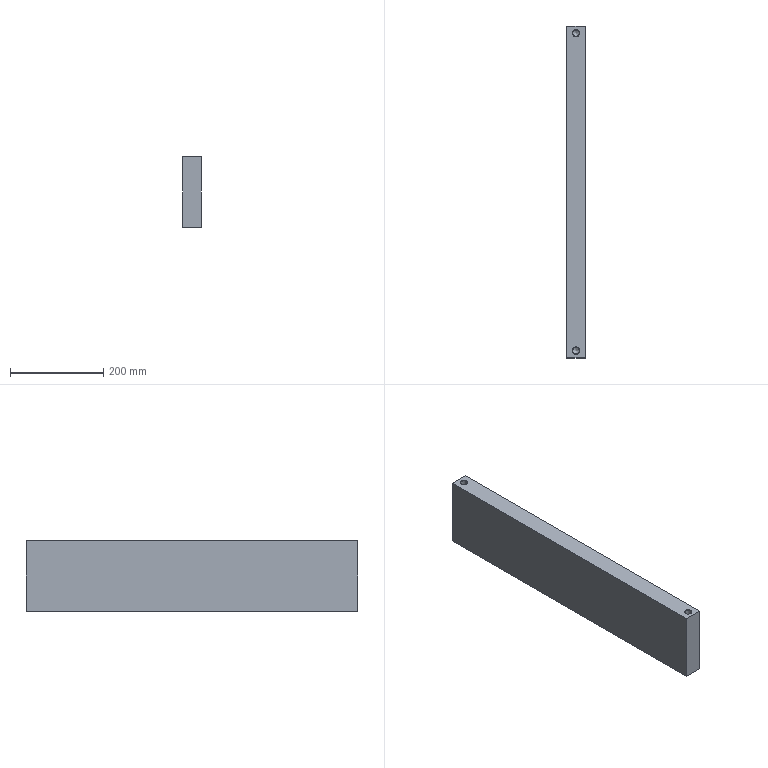Part | NX | features solid 2 | 1 solid | 18 faces | box 40 x 710 x 151.131 mm | volume 4263448 mm3 | cone 8 | plane 6 | cylinder 4 | commonest cylinder face diameters 14 x4
STEP:
#1=CARTESIAN_POINT('',(1264.977,357.095,246.13));
#2=VERTEX_POINT('',#1);
#3=CARTESIAN_POINT('',(1264.977,-352.905,246.13));
#4=VERTEX_POINT('',#3);
#5=CARTESIAN_POINT('',(1264.977,2.095,246.13));
#6=DIRECTION('',(0.,-1.,0.));
#7=VECTOR('',#6,1000.);
#8=LINE('',#5,#7);
#9=EDGE_CURVE('',#2,#4,#8,.T.);
#10=ORIENTED_EDGE('',*,*,#9,.F.);
#11=CARTESIAN_POINT('',(1264.977,357.095,94.999));
#12=VERTEX_POINT('',#11);
#13=CARTESIAN_POINT('',(1264.977,357.095,289.999));
#14=DIRECTION('',(0.,0.,1.));
#15=VECTOR('',#14,1000.);
#16=LINE('',#13,#15);
#17=EDGE_CURVE('',#12,#2,#16,.T.);
#18=ORIENTED_EDGE('',*,*,#17,.F.);
#19=CARTESIAN_POINT('',(1264.977,-352.905,94.999));
#20=VERTEX_POINT('',#19);
#21=CARTESIAN_POINT('',(1264.977,2.095,94.999));
#22=DIRECTION('',(0.,1.,0.));
#23=VECTOR('',#22,1000.);
#24=LINE('',#21,#23);
#25=EDGE_CURVE('',#12,#20,#24,.F.);
#26=ORIENTED_EDGE('',*,*,#25,.T.);
#27=CARTESIAN_POINT('',(1264.977,-352.905,289.999));
#28=DIRECTION('',(0.,0.,-1.));
#29=VECTOR('',#28,1000.);
#30=LINE('',#27,#29);
#31=EDGE_CURVE('',#4,#20,#30,.T.);
#32=ORIENTED_EDGE('',*,*,#31,.F.);
#33=EDGE_LOOP('',(#10,#18,#26,#32));
#34=FACE_BOUND('',#33,.T.);
#35=CARTESIAN_POINT('',(1264.977,2.095,159.999));
#36=DIRECTION('',(-1.,0.,0.));
#37=DIRECTION('',(0.,0.,-1.));
#38=AXIS2_PLACEMENT_3D('',#35,#36,#37);
#39=PLANE('',#38);
#40=ADVANCED_FACE('',(#34),#39,.T.);
#41=CARTESIAN_POINT('',(1304.977,-352.905,94.999));
#42=VERTEX_POINT('',#41);
#43=CARTESIAN_POINT('',(1304.977,357.095,94.999));
#44=VERTEX_POINT('',#43);
#45=CARTESIAN_POINT('',(1304.977,2.095,94.999));
#46=DIRECTION('',(0.,-1.,0.));
#47=VECTOR('',#46,1000.);
#48=LINE('',#45,#47);
#49=EDGE_CURVE('',#42,#44,#48,.F.);
#50=ORIENTED_EDGE('',*,*,#49,.T.);
#51=CARTESIAN_POINT('',(1304.977,357.095,246.13));
#52=VERTEX_POINT('',#51);
#53=CARTESIAN_POINT('',(1304.977,357.095,289.999));
#54=DIRECTION('',(0.,0.,-1.));
#55=VECTOR('',#54,1000.);
#56=LINE('',#53,#55);
#57=EDGE_CURVE('',#52,#44,#56,.T.);
#58=ORIENTED_EDGE('',*,*,#57,.F.);
#59=CARTESIAN_POINT('',(1304.977,-352.905,246.13));
#60=VERTEX_POINT('',#59);
#61=CARTESIAN_POINT('',(1304.977,2.095,246.13));
#62=DIRECTION('',(0.,1.,0.));
#63=VECTOR('',#62,1000.);
#64=LINE('',#61,#63);
#65=EDGE_CURVE('',#60,#52,#64,.T.);
#66=ORIENTED_EDGE('',*,*,#65,.F.);
#67=CARTESIAN_POINT('',(1304.977,-352.905,159.999));
#68=DIRECTION('',(0.,0.,-1.));
#69=VECTOR('',#68,1000.);
#70=LINE('',#67,#69);
#71=EDGE_CURVE('',#60,#42,#70,.T.);
#72=ORIENTED_EDGE('',*,*,#71,.T.);
#73=EDGE_LOOP('',(#50,#58,#66,#72));
#74=FACE_BOUND('',#73,.T.);
#75=CARTESIAN_POINT('',(1304.977,2.095,159.999));
#76=DIRECTION('',(1.,0.,0.));
#77=DIRECTION('',(0.,0.,1.));
#78=AXIS2_PLACEMENT_3D('',#75,#76,#77);
#79=PLANE('',#78);
#80=ADVANCED_FACE('',(#74),#79,.T.);
#81=CARTESIAN_POINT('',(1278.977,203.595,94.999));
#82=VERTEX_POINT('',#81);
#83=CARTESIAN_POINT('',(1286.977,203.595,94.999));
#84=DIRECTION('',(0.,0.,-1.));
#85=DIRECTION('',(-1.,0.,0.));
#86=AXIS2_PLACEMENT_3D('',#83,#84,#85);
#87=CIRCLE('',#86,8.);
#88=EDGE_CURVE('',#82,#82,#87,.F.);
#89=ORIENTED_EDGE('',*,*,#88,.T.);
#90=EDGE_LOOP('',(#89));
#91=FACE_BOUND('',#90,.T.);
#92=CARTESIAN_POINT('',(1278.977,-199.405,94.999));
#93=VERTEX_POINT('',#92);
#94=CARTESIAN_POINT('',(1286.977,-199.405,94.999));
#95=DIRECTION('',(0.,0.,-1.));
#96=DIRECTION('',(-1.,0.,0.));
#97=AXIS2_PLACEMENT_3D('',#94,#95,#96);
#98=CIRCLE('',#97,8.);
#99=EDGE_CURVE('',#93,#93,#98,.F.);
#100=ORIENTED_EDGE('',*,*,#99,.T.);
#101=EDGE_LOOP('',(#100));
#102=FACE_BOUND('',#101,.T.);
#103=CARTESIAN_POINT('',(1469.955,357.095,94.999));
#104=DIRECTION('',(1.,0.,0.));
#105=VECTOR('',#104,1000.);
#106=LINE('',#103,#105);
#107=EDGE_CURVE('',#44,#12,#106,.F.);
#108=ORIENTED_EDGE('',*,*,#107,.F.);
#109=ORIENTED_EDGE('',*,*,#49,.F.);
#110=CARTESIAN_POINT('',(1469.955,-352.905,94.999));
#111=DIRECTION('',(-1.,0.,0.));
#112=VECTOR('',#111,1000.);
#113=LINE('',#110,#112);
#114=EDGE_CURVE('',#20,#42,#113,.F.);
#115=ORIENTED_EDGE('',*,*,#114,.F.);
#116=ORIENTED_EDGE('',*,*,#25,.F.);
#117=EDGE_LOOP('',(#108,#109,#115,#116));
#118=FACE_BOUND('',#117,.T.);
#119=CARTESIAN_POINT('',(1469.955,6.94,94.999));
#120=DIRECTION('',(0.,0.,-1.));
#121=DIRECTION('',(-1.,0.,0.));
#122=AXIS2_PLACEMENT_3D('',#119,#120,#121);
#123=PLANE('',#122);
#124=ADVANCED_FACE('',(#91,#102,#118),#123,.T.);
#125=CARTESIAN_POINT('',(1276.977,-337.405,246.13));
#126=VERTEX_POINT('',#125);
#127=CARTESIAN_POINT('',(1284.977,-337.405,246.13));
#128=DIRECTION('',(0.,0.,-1.));
#129=DIRECTION('',(-1.,0.,0.));
#130=AXIS2_PLACEMENT_3D('',#127,#128,#129);
#131=CIRCLE('',#130,8.);
#132=EDGE_CURVE('',#126,#126,#131,.T.);
#133=ORIENTED_EDGE('',*,*,#132,.T.);
#134=EDGE_LOOP('',(#133));
#135=FACE_BOUND('',#134,.T.);
#136=CARTESIAN_POINT('',(1276.977,341.595,246.13));
#137=VERTEX_POINT('',#136);
#138=CARTESIAN_POINT('',(1284.977,341.595,246.13));
#139=DIRECTION('',(0.,0.,-1.));
#140=DIRECTION('',(-1.,0.,0.));
#141=AXIS2_PLACEMENT_3D('',#138,#139,#140);
#142=CIRCLE('',#141,8.);
#143=EDGE_CURVE('',#137,#137,#142,.T.);
#144=ORIENTED_EDGE('',*,*,#143,.T.);
#145=EDGE_LOOP('',(#144));
#146=FACE_BOUND('',#145,.T.);
#147=CARTESIAN_POINT('',(3474.955,357.095,246.13));
#148=DIRECTION('',(1.,0.,0.));
#149=VECTOR('',#148,1000.);
#150=LINE('',#147,#149);
#151=EDGE_CURVE('',#2,#52,#150,.T.);
#152=ORIENTED_EDGE('',*,*,#151,.F.);
#153=ORIENTED_EDGE('',*,*,#9,.T.);
#154=CARTESIAN_POINT('',(3474.955,-352.905,246.13));
#155=DIRECTION('',(-1.,0.,0.));
#156=VECTOR('',#155,1000.);
#157=LINE('',#154,#156);
#158=EDGE_CURVE('',#60,#4,#157,.T.);
#159=ORIENTED_EDGE('',*,*,#158,.F.);
#160=ORIENTED_EDGE('',*,*,#65,.T.);
#161=EDGE_LOOP('',(#152,#153,#159,#160));
#162=FACE_BOUND('',#161,.T.);
#163=CARTESIAN_POINT('',(3474.955,4.191,246.13));
#164=DIRECTION('',(0.,0.,-1.));
#165=DIRECTION('',(1.,0.,0.));
#166=AXIS2_PLACEMENT_3D('',#163,#164,#165);
#167=PLANE('',#166);
#168=ADVANCED_FACE('',(#135,#146,#162),#167,.F.);
#169=ORIENTED_EDGE('',*,*,#158,.T.);
#170=ORIENTED_EDGE('',*,*,#31,.T.);
#171=ORIENTED_EDGE('',*,*,#114,.T.);
#172=ORIENTED_EDGE('',*,*,#71,.F.);
#173=EDGE_LOOP('',(#169,#170,#171,#172));
#174=FACE_BOUND('',#173,.T.);
#175=CARTESIAN_POINT('',(1344.977,-352.905,289.999));
#176=DIRECTION('',(0.,-1.,0.));
#177=DIRECTION('',(0.,0.,-1.));
#178=AXIS2_PLACEMENT_3D('',#175,#176,#177);
#179=PLANE('',#178);
#180=ADVANCED_FACE('',(#174),#179,.T.);
#181=ORIENTED_EDGE('',*,*,#151,.T.);
#182=ORIENTED_EDGE('',*,*,#57,.T.);
#183=ORIENTED_EDGE('',*,*,#107,.T.);
#184=ORIENTED_EDGE('',*,*,#17,.T.);
#185=EDGE_LOOP('',(#181,#182,#183,#184));
#186=FACE_BOUND('',#185,.T.);
#187=CARTESIAN_POINT('',(1344.977,357.095,289.999));
#188=DIRECTION('',(0.,1.,0.));
#189=DIRECTION('',(0.,0.,1.));
#190=AXIS2_PLACEMENT_3D('',#187,#188,#189);
#191=PLANE('',#190);
#192=ADVANCED_FACE('',(#186),#191,.T.);
#193=CARTESIAN_POINT('',(1293.977,-199.405,139.999));
#194=VERTEX_POINT('',#193);
#195=CARTESIAN_POINT('',(1286.977,-199.405,139.999));
#196=DIRECTION('',(0.,0.,1.));
#197=DIRECTION('',(1.,0.,0.));
#198=AXIS2_PLACEMENT_3D('',#195,#196,#197);
#199=CIRCLE('',#198,7.);
#200=EDGE_CURVE('',#194,#194,#199,.F.);
#201=ORIENTED_EDGE('',*,*,#200,.T.);
#202=EDGE_LOOP('',(#201));
#203=FACE_BOUND('',#202,.T.);
#204=CARTESIAN_POINT('',(1286.977,-199.405,144.205));
#205=VERTEX_POINT('',#204);
#206=VERTEX_LOOP('',#205);
#207=FACE_BOUND('',#206,.T.);
#208=CARTESIAN_POINT('',(1286.977,-199.405,139.999));
#209=DIRECTION('',(0.,0.,-1.));
#210=DIRECTION('',(-1.,0.,0.));
#211=AXIS2_PLACEMENT_3D('',#208,#209,#210);
#212=CONICAL_SURFACE('',#211,7.,1.03);
#213=ADVANCED_FACE('',(#203,#207),#212,.F.);
#214=CARTESIAN_POINT('',(1293.977,-199.405,95.999));
#215=VERTEX_POINT('',#214);
#216=CARTESIAN_POINT('',(1286.977,-199.405,95.999));
#217=DIRECTION('',(0.,0.,1.));
#218=DIRECTION('',(1.,0.,0.));
#219=AXIS2_PLACEMENT_3D('',#216,#217,#218);
#220=CIRCLE('',#219,7.);
#221=EDGE_CURVE('',#215,#215,#220,.F.);
#222=ORIENTED_EDGE('',*,*,#221,.T.);
#223=EDGE_LOOP('',(#222));
#224=FACE_BOUND('',#223,.T.);
#225=ORIENTED_EDGE('',*,*,#200,.F.);
#226=EDGE_LOOP('',(#225));
#227=FACE_BOUND('',#226,.T.);
#228=CARTESIAN_POINT('',(1286.977,-199.405,94.999));
#229=DIRECTION('',(0.,0.,1.));
#230=DIRECTION('',(1.,0.,0.));
#231=AXIS2_PLACEMENT_3D('',#228,#229,#230);
#232=CYLINDRICAL_SURFACE('',#231,7.);
#233=ADVANCED_FACE('',(#224,#227),#232,.F.);
#234=ORIENTED_EDGE('',*,*,#221,.F.);
#235=EDGE_LOOP('',(#234));
#236=FACE_BOUND('',#235,.T.);
#237=ORIENTED_EDGE('',*,*,#99,.F.);
#238=EDGE_LOOP('',(#237));
#239=FACE_BOUND('',#238,.T.);
#240=CARTESIAN_POINT('',(1286.977,-199.405,94.999));
#241=DIRECTION('',(0.,0.,-1.));
#242=DIRECTION('',(-1.,0.,0.));
#243=AXIS2_PLACEMENT_3D('',#240,#241,#242);
#244=CONICAL_SURFACE('',#243,8.,0.7854);
#245=ADVANCED_FACE('',(#236,#239),#244,.F.);
#246=CARTESIAN_POINT('',(1293.977,203.595,139.999));
#247=VERTEX_POINT('',#246);
#248=CARTESIAN_POINT('',(1286.977,203.595,139.999));
#249=DIRECTION('',(0.,0.,1.));
#250=DIRECTION('',(1.,0.,0.));
#251=AXIS2_PLACEMENT_3D('',#248,#249,#250);
#252=CIRCLE('',#251,7.);
#253=EDGE_CURVE('',#247,#247,#252,.F.);
#254=ORIENTED_EDGE('',*,*,#253,.T.);
#255=EDGE_LOOP('',(#254));
#256=FACE_BOUND('',#255,.T.);
#257=CARTESIAN_POINT('',(1286.977,203.595,144.205));
#258=VERTEX_POINT('',#257);
#259=VERTEX_LOOP('',#258);
#260=FACE_BOUND('',#259,.T.);
#261=CARTESIAN_POINT('',(1286.977,203.595,139.999));
#262=DIRECTION('',(0.,0.,-1.));
#263=DIRECTION('',(-1.,0.,0.));
#264=AXIS2_PLACEMENT_3D('',#261,#262,#263);
#265=CONICAL_SURFACE('',#264,7.,1.03);
#266=ADVANCED_FACE('',(#256,#260),#265,.F.);
#267=CARTESIAN_POINT('',(1293.977,203.595,95.999));
#268=VERTEX_POINT('',#267);
#269=CARTESIAN_POINT('',(1286.977,203.595,95.999));
#270=DIRECTION('',(0.,0.,1.));
#271=DIRECTION('',(1.,0.,0.));
#272=AXIS2_PLACEMENT_3D('',#269,#270,#271);
#273=CIRCLE('',#272,7.);
#274=EDGE_CURVE('',#268,#268,#273,.F.);
#275=ORIENTED_EDGE('',*,*,#274,.T.);
#276=EDGE_LOOP('',(#275));
#277=FACE_BOUND('',#276,.T.);
#278=ORIENTED_EDGE('',*,*,#253,.F.);
#279=EDGE_LOOP('',(#278));
#280=FACE_BOUND('',#279,.T.);
#281=CARTESIAN_POINT('',(1286.977,203.595,94.999));
#282=DIRECTION('',(0.,0.,1.));
#283=DIRECTION('',(1.,0.,0.));
#284=AXIS2_PLACEMENT_3D('',#281,#282,#283);
#285=CYLINDRICAL_SURFACE('',#284,7.);
#286=ADVANCED_FACE('',(#277,#280),#285,.F.);
#287=ORIENTED_EDGE('',*,*,#274,.F.);
#288=EDGE_LOOP('',(#287));
#289=FACE_BOUND('',#288,.T.);
#290=ORIENTED_EDGE('',*,*,#88,.F.);
#291=EDGE_LOOP('',(#290));
#292=FACE_BOUND('',#291,.T.);
#293=CARTESIAN_POINT('',(1286.977,203.595,94.999));
#294=DIRECTION('',(0.,0.,-1.));
#295=DIRECTION('',(-1.,0.,0.));
#296=AXIS2_PLACEMENT_3D('',#293,#294,#295);
#297=CONICAL_SURFACE('',#296,8.,0.7854);
#298=ADVANCED_FACE('',(#289,#292),#297,.F.);
#299=CARTESIAN_POINT('',(1277.977,341.595,201.13));
#300=VERTEX_POINT('',#299);
#301=CARTESIAN_POINT('',(1284.977,341.595,201.13));
#302=DIRECTION('',(0.,0.,-1.));
#303=DIRECTION('',(-1.,0.,0.));
#304=AXIS2_PLACEMENT_3D('',#301,#302,#303);
#305=CIRCLE('',#304,7.);
#306=EDGE_CURVE('',#300,#300,#305,.F.);
#307=ORIENTED_EDGE('',*,*,#306,.T.);
#308=EDGE_LOOP('',(#307));
#309=FACE_BOUND('',#308,.T.);
#310=CARTESIAN_POINT('',(1284.977,341.595,196.924));
#311=VERTEX_POINT('',#310);
#312=VERTEX_LOOP('',#311);
#313=FACE_BOUND('',#312,.T.);
#314=CARTESIAN_POINT('',(1284.977,341.595,201.13));
#315=DIRECTION('',(0.,0.,1.));
#316=DIRECTION('',(1.,0.,0.));
#317=AXIS2_PLACEMENT_3D('',#314,#315,#316);
#318=CONICAL_SURFACE('',#317,7.,1.03);
#319=ADVANCED_FACE('',(#309,#313),#318,.F.);
#320=CARTESIAN_POINT('',(1277.977,341.595,245.13));
#321=VERTEX_POINT('',#320);
#322=CARTESIAN_POINT('',(1284.977,341.595,245.13));
#323=DIRECTION('',(0.,0.,-1.));
#324=DIRECTION('',(-1.,0.,0.));
#325=AXIS2_PLACEMENT_3D('',#322,#323,#324);
#326=CIRCLE('',#325,7.);
#327=EDGE_CURVE('',#321,#321,#326,.F.);
#328=ORIENTED_EDGE('',*,*,#327,.T.);
#329=EDGE_LOOP('',(#328));
#330=FACE_BOUND('',#329,.T.);
#331=ORIENTED_EDGE('',*,*,#306,.F.);
#332=EDGE_LOOP('',(#331));
#333=FACE_BOUND('',#332,.T.);
#334=CARTESIAN_POINT('',(1284.977,341.595,246.13));
#335=DIRECTION('',(0.,0.,-1.));
#336=DIRECTION('',(-1.,0.,0.));
#337=AXIS2_PLACEMENT_3D('',#334,#335,#336);
#338=CYLINDRICAL_SURFACE('',#337,7.);
#339=ADVANCED_FACE('',(#330,#333),#338,.F.);
#340=ORIENTED_EDGE('',*,*,#327,.F.);
#341=EDGE_LOOP('',(#340));
#342=FACE_BOUND('',#341,.T.);
#343=ORIENTED_EDGE('',*,*,#143,.F.);
#344=EDGE_LOOP('',(#343));
#345=FACE_BOUND('',#344,.T.);
#346=CARTESIAN_POINT('',(1284.977,341.595,246.13));
#347=DIRECTION('',(0.,0.,1.));
#348=DIRECTION('',(1.,0.,0.));
#349=AXIS2_PLACEMENT_3D('',#346,#347,#348);
#350=CONICAL_SURFACE('',#349,8.,0.7854);
#351=ADVANCED_FACE('',(#342,#345),#350,.F.);
#352=CARTESIAN_POINT('',(1277.977,-337.405,201.13));
#353=VERTEX_POINT('',#352);
#354=CARTESIAN_POINT('',(1284.977,-337.405,201.13));
#355=DIRECTION('',(0.,0.,-1.));
#356=DIRECTION('',(-1.,0.,0.));
#357=AXIS2_PLACEMENT_3D('',#354,#355,#356);
#358=CIRCLE('',#357,7.);
#359=EDGE_CURVE('',#353,#353,#358,.F.);
#360=ORIENTED_EDGE('',*,*,#359,.T.);
#361=EDGE_LOOP('',(#360));
#362=FACE_BOUND('',#361,.T.);
#363=CARTESIAN_POINT('',(1284.977,-337.405,196.924));
#364=VERTEX_POINT('',#363);
#365=VERTEX_LOOP('',#364);
#366=FACE_BOUND('',#365,.T.);
#367=CARTESIAN_POINT('',(1284.977,-337.405,201.13));
#368=DIRECTION('',(0.,0.,1.));
#369=DIRECTION('',(1.,0.,0.));
#370=AXIS2_PLACEMENT_3D('',#367,#368,#369);
#371=CONICAL_SURFACE('',#370,7.,1.03);
#372=ADVANCED_FACE('',(#362,#366),#371,.F.);
#373=CARTESIAN_POINT('',(1277.977,-337.405,245.13));
#374=VERTEX_POINT('',#373);
#375=CARTESIAN_POINT('',(1284.977,-337.405,245.13));
#376=DIRECTION('',(0.,0.,-1.));
#377=DIRECTION('',(-1.,0.,0.));
#378=AXIS2_PLACEMENT_3D('',#375,#376,#377);
#379=CIRCLE('',#378,7.);
#380=EDGE_CURVE('',#374,#374,#379,.F.);
#381=ORIENTED_EDGE('',*,*,#380,.T.);
#382=EDGE_LOOP('',(#381));
#383=FACE_BOUND('',#382,.T.);
#384=ORIENTED_EDGE('',*,*,#359,.F.);
#385=EDGE_LOOP('',(#384));
#386=FACE_BOUND('',#385,.T.);
#387=CARTESIAN_POINT('',(1284.977,-337.405,246.13));
#388=DIRECTION('',(0.,0.,-1.));
#389=DIRECTION('',(-1.,0.,0.));
#390=AXIS2_PLACEMENT_3D('',#387,#388,#389);
#391=CYLINDRICAL_SURFACE('',#390,7.);
#392=ADVANCED_FACE('',(#383,#386),#391,.F.);
#393=ORIENTED_EDGE('',*,*,#380,.F.);
#394=EDGE_LOOP('',(#393));
#395=FACE_BOUND('',#394,.T.);
#396=ORIENTED_EDGE('',*,*,#132,.F.);
#397=EDGE_LOOP('',(#396));
#398=FACE_BOUND('',#397,.T.);
#399=CARTESIAN_POINT('',(1284.977,-337.405,246.13));
#400=DIRECTION('',(0.,0.,1.));
#401=DIRECTION('',(1.,0.,0.));
#402=AXIS2_PLACEMENT_3D('',#399,#400,#401);
#403=CONICAL_SURFACE('',#402,8.,0.7854);
#404=ADVANCED_FACE('',(#395,#398),#403,.F.);
#405=CLOSED_SHELL('',(#40,#80,#124,#168,#180,#192,#213,#233,#245,#266,#286,#298,#319,#339,#351,#372,#392,#404));
#406=MANIFOLD_SOLID_BREP('',#405);
#407=(LENGTH_UNIT()NAMED_UNIT(*)SI_UNIT(.MILLI.,.METRE.));
#408=UNCERTAINTY_MEASURE_WITH_UNIT(LENGTH_MEASURE(0.00001),#407,'','');
#409=(NAMED_UNIT(*)PLANE_ANGLE_UNIT()SI_UNIT($,.RADIAN.));
#410=(NAMED_UNIT(*)SI_UNIT($,.STERADIAN.)SOLID_ANGLE_UNIT());
#411=(GEOMETRIC_REPRESENTATION_CONTEXT(3)GLOBAL_UNCERTAINTY_ASSIGNED_CONTEXT((#408))GLOBAL_UNIT_ASSIGNED_CONTEXT((#407,#409,#410))REPRESENTATION_CONTEXT('',''));
#412=ADVANCED_BREP_SHAPE_REPRESENTATION('',(#406),#411);